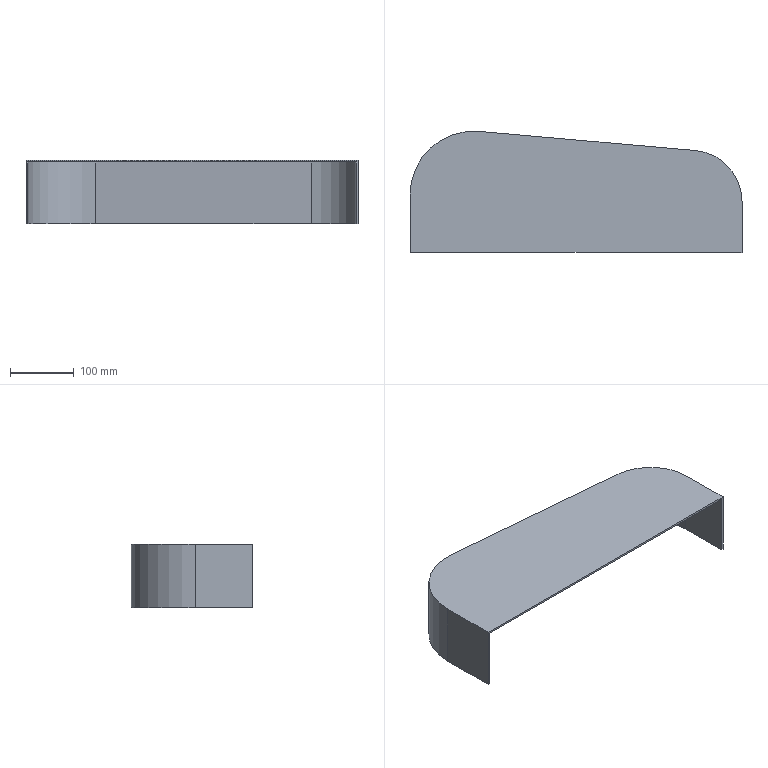Part | SolidWorks | features FlatPattern 1, SMBaseFlange 1, SheetMetal 1, Shell 1 | 1 solid | 14 faces | box 520 x 190 x 100 mm | volume 493401 mm3 | plane 10 | cylinder 4 | commonest cylinder face diameters 154 x1 160 x1 194 x1 200 x1
STEP:
#1=CARTESIAN_POINT('',(-100.,0.,-100.));
#2=VERTEX_POINT('',#1);
#3=CARTESIAN_POINT('',(-97.,0.,-100.));
#4=VERTEX_POINT('',#3);
#5=CARTESIAN_POINT('',(-100.,0.,-100.));
#6=DIRECTION('',(1.,0.,0.));
#7=VECTOR('',#6,1000.);
#8=LINE('',#5,#7);
#9=EDGE_CURVE('',#2,#4,#8,.T.);
#10=ORIENTED_EDGE('',*,*,#9,.T.);
#11=CARTESIAN_POINT('',(-97.,0.,-3.));
#12=VERTEX_POINT('',#11);
#13=CARTESIAN_POINT('',(-97.,0.,-100.));
#14=DIRECTION('',(0.,0.,1.));
#15=VECTOR('',#14,1000.);
#16=LINE('',#13,#15);
#17=EDGE_CURVE('',#4,#12,#16,.T.);
#18=ORIENTED_EDGE('',*,*,#17,.T.);
#19=CARTESIAN_POINT('',(417.,0.,-3.));
#20=VERTEX_POINT('',#19);
#21=CARTESIAN_POINT('',(0.,0.,-3.));
#22=DIRECTION('',(1.,0.,0.));
#23=VECTOR('',#22,1000.);
#24=LINE('',#21,#23);
#25=EDGE_CURVE('',#12,#20,#24,.T.);
#26=ORIENTED_EDGE('',*,*,#25,.T.);
#27=CARTESIAN_POINT('',(417.,0.,-100.));
#28=VERTEX_POINT('',#27);
#29=CARTESIAN_POINT('',(417.,0.,-100.));
#30=DIRECTION('',(0.,0.,1.));
#31=VECTOR('',#30,1000.);
#32=LINE('',#29,#31);
#33=EDGE_CURVE('',#28,#20,#32,.T.);
#34=ORIENTED_EDGE('',*,*,#33,.F.);
#35=CARTESIAN_POINT('',(420.,0.,-100.));
#36=VERTEX_POINT('',#35);
#37=CARTESIAN_POINT('',(-100.,0.,-100.));
#38=DIRECTION('',(1.,0.,0.));
#39=VECTOR('',#38,1000.);
#40=LINE('',#37,#39);
#41=EDGE_CURVE('',#28,#36,#40,.T.);
#42=ORIENTED_EDGE('',*,*,#41,.T.);
#43=CARTESIAN_POINT('',(420.,0.,0.));
#44=VERTEX_POINT('',#43);
#45=CARTESIAN_POINT('',(420.,0.,-100.));
#46=DIRECTION('',(0.,0.,1.));
#47=VECTOR('',#46,1000.);
#48=LINE('',#45,#47);
#49=EDGE_CURVE('',#36,#44,#48,.T.);
#50=ORIENTED_EDGE('',*,*,#49,.T.);
#51=CARTESIAN_POINT('',(-100.,0.,0.));
#52=VERTEX_POINT('',#51);
#53=CARTESIAN_POINT('',(-100.,0.,0.));
#54=DIRECTION('',(1.,0.,0.));
#55=VECTOR('',#54,1000.);
#56=LINE('',#53,#55);
#57=EDGE_CURVE('',#52,#44,#56,.T.);
#58=ORIENTED_EDGE('',*,*,#57,.F.);
#59=CARTESIAN_POINT('',(-100.,0.,-100.));
#60=DIRECTION('',(0.,0.,1.));
#61=VECTOR('',#60,1000.);
#62=LINE('',#59,#61);
#63=EDGE_CURVE('',#2,#52,#62,.T.);
#64=ORIENTED_EDGE('',*,*,#63,.F.);
#65=EDGE_LOOP('',(#10,#18,#26,#34,#42,#50,#58,#64));
#66=FACE_OUTER_BOUND('',#65,.T.);
#67=CARTESIAN_POINT('',(-100.,0.,-100.));
#68=DIRECTION('',(0.,-1.,0.));
#69=DIRECTION('',(1.,0.,0.));
#70=AXIS2_PLACEMENT_3D('',#67,#68,#69);
#71=PLANE('',#70);
#72=ADVANCED_FACE('',(#66),#71,.T.);
#73=CARTESIAN_POINT('',(8.812,189.611,0.));
#74=VERTEX_POINT('',#73);
#75=CARTESIAN_POINT('',(-100.,90.,0.));
#76=VERTEX_POINT('',#75);
#77=CARTESIAN_POINT('',(0.,90.,0.));
#78=DIRECTION('',(0.,0.,1.));
#79=DIRECTION('',(1.,0.,0.));
#80=AXIS2_PLACEMENT_3D('',#77,#78,#79);
#81=CIRCLE('',#80,100.);
#82=EDGE_CURVE('',#74,#76,#81,.T.);
#83=ORIENTED_EDGE('',*,*,#82,.F.);
#84=CARTESIAN_POINT('',(8.812,189.611,-100.));
#85=VERTEX_POINT('',#84);
#86=CARTESIAN_POINT('',(8.812,189.611,-100.));
#87=DIRECTION('',(0.,0.,1.));
#88=VECTOR('',#87,1000.);
#89=LINE('',#86,#88);
#90=EDGE_CURVE('',#85,#74,#89,.T.);
#91=ORIENTED_EDGE('',*,*,#90,.F.);
#92=CARTESIAN_POINT('',(-100.,90.,-100.));
#93=VERTEX_POINT('',#92);
#94=CARTESIAN_POINT('',(0.,90.,-100.));
#95=DIRECTION('',(0.,0.,1.));
#96=DIRECTION('',(1.,0.,0.));
#97=AXIS2_PLACEMENT_3D('',#94,#95,#96);
#98=CIRCLE('',#97,100.);
#99=EDGE_CURVE('',#85,#93,#98,.T.);
#100=ORIENTED_EDGE('',*,*,#99,.T.);
#101=CARTESIAN_POINT('',(-100.,90.,-100.));
#102=DIRECTION('',(0.,0.,1.));
#103=VECTOR('',#102,1000.);
#104=LINE('',#101,#103);
#105=EDGE_CURVE('',#93,#76,#104,.T.);
#106=ORIENTED_EDGE('',*,*,#105,.T.);
#107=EDGE_LOOP('',(#83,#91,#100,#106));
#108=FACE_OUTER_BOUND('',#107,.T.);
#109=CARTESIAN_POINT('',(0.,90.,-100.));
#110=DIRECTION('',(0.,0.,1.));
#111=DIRECTION('',(1.,0.,0.));
#112=AXIS2_PLACEMENT_3D('',#109,#110,#111);
#113=CYLINDRICAL_SURFACE('',#112,100.);
#114=ADVANCED_FACE('',(#108),#113,.T.);
#115=CARTESIAN_POINT('',(347.05,159.689,0.));
#116=VERTEX_POINT('',#115);
#117=CARTESIAN_POINT('',(8.812,189.611,0.));
#118=DIRECTION('',(-0.9961,0.08812,0.));
#119=VECTOR('',#118,1000.);
#120=LINE('',#117,#119);
#121=EDGE_CURVE('',#116,#74,#120,.T.);
#122=ORIENTED_EDGE('',*,*,#121,.F.);
#123=CARTESIAN_POINT('',(347.05,159.689,-100.));
#124=VERTEX_POINT('',#123);
#125=CARTESIAN_POINT('',(347.05,159.689,-100.));
#126=DIRECTION('',(0.,0.,1.));
#127=VECTOR('',#126,1000.);
#128=LINE('',#125,#127);
#129=EDGE_CURVE('',#124,#116,#128,.T.);
#130=ORIENTED_EDGE('',*,*,#129,.F.);
#131=CARTESIAN_POINT('',(8.812,189.611,-100.));
#132=DIRECTION('',(-0.9961,0.08812,0.));
#133=VECTOR('',#132,1000.);
#134=LINE('',#131,#133);
#135=EDGE_CURVE('',#124,#85,#134,.T.);
#136=ORIENTED_EDGE('',*,*,#135,.T.);
#137=ORIENTED_EDGE('',*,*,#90,.T.);
#138=EDGE_LOOP('',(#122,#130,#136,#137));
#139=FACE_OUTER_BOUND('',#138,.T.);
#140=CARTESIAN_POINT('',(8.812,189.611,-100.));
#141=DIRECTION('',(0.08812,0.9961,0.));
#142=DIRECTION('',(-0.9961,0.08812,0.));
#143=AXIS2_PLACEMENT_3D('',#140,#141,#142);
#144=PLANE('',#143);
#145=ADVANCED_FACE('',(#139),#144,.T.);
#146=CARTESIAN_POINT('',(420.,80.,0.));
#147=VERTEX_POINT('',#146);
#148=CARTESIAN_POINT('',(340.,80.,0.));
#149=DIRECTION('',(0.,0.,1.));
#150=DIRECTION('',(1.,0.,0.));
#151=AXIS2_PLACEMENT_3D('',#148,#149,#150);
#152=CIRCLE('',#151,80.);
#153=EDGE_CURVE('',#147,#116,#152,.T.);
#154=ORIENTED_EDGE('',*,*,#153,.F.);
#155=CARTESIAN_POINT('',(420.,80.,-100.));
#156=VERTEX_POINT('',#155);
#157=CARTESIAN_POINT('',(420.,80.,-100.));
#158=DIRECTION('',(0.,0.,1.));
#159=VECTOR('',#158,1000.);
#160=LINE('',#157,#159);
#161=EDGE_CURVE('',#156,#147,#160,.T.);
#162=ORIENTED_EDGE('',*,*,#161,.F.);
#163=CARTESIAN_POINT('',(340.,80.,-100.));
#164=DIRECTION('',(0.,0.,1.));
#165=DIRECTION('',(1.,0.,0.));
#166=AXIS2_PLACEMENT_3D('',#163,#164,#165);
#167=CIRCLE('',#166,80.);
#168=EDGE_CURVE('',#156,#124,#167,.T.);
#169=ORIENTED_EDGE('',*,*,#168,.T.);
#170=ORIENTED_EDGE('',*,*,#129,.T.);
#171=EDGE_LOOP('',(#154,#162,#169,#170));
#172=FACE_OUTER_BOUND('',#171,.T.);
#173=CARTESIAN_POINT('',(340.,80.,-100.));
#174=DIRECTION('',(0.,0.,1.));
#175=DIRECTION('',(1.,0.,0.));
#176=AXIS2_PLACEMENT_3D('',#173,#174,#175);
#177=CYLINDRICAL_SURFACE('',#176,80.);
#178=ADVANCED_FACE('',(#172),#177,.T.);
#179=CARTESIAN_POINT('',(420.,80.,0.));
#180=DIRECTION('',(0.,1.,0.));
#181=VECTOR('',#180,1000.);
#182=LINE('',#179,#181);
#183=EDGE_CURVE('',#44,#147,#182,.T.);
#184=ORIENTED_EDGE('',*,*,#183,.F.);
#185=ORIENTED_EDGE('',*,*,#49,.F.);
#186=CARTESIAN_POINT('',(420.,80.,-100.));
#187=DIRECTION('',(0.,1.,0.));
#188=VECTOR('',#187,1000.);
#189=LINE('',#186,#188);
#190=EDGE_CURVE('',#36,#156,#189,.T.);
#191=ORIENTED_EDGE('',*,*,#190,.T.);
#192=ORIENTED_EDGE('',*,*,#161,.T.);
#193=EDGE_LOOP('',(#184,#185,#191,#192));
#194=FACE_OUTER_BOUND('',#193,.T.);
#195=CARTESIAN_POINT('',(420.,80.,-100.));
#196=DIRECTION('',(1.,0.,0.));
#197=DIRECTION('',(0.,0.,-1.));
#198=AXIS2_PLACEMENT_3D('',#195,#196,#197);
#199=PLANE('',#198);
#200=ADVANCED_FACE('',(#194),#199,.T.);
#201=CARTESIAN_POINT('',(-100.,90.,0.));
#202=DIRECTION('',(0.,-1.,0.));
#203=VECTOR('',#202,1000.);
#204=LINE('',#201,#203);
#205=EDGE_CURVE('',#76,#52,#204,.T.);
#206=ORIENTED_EDGE('',*,*,#205,.F.);
#207=ORIENTED_EDGE('',*,*,#105,.F.);
#208=CARTESIAN_POINT('',(-100.,90.,-100.));
#209=DIRECTION('',(0.,-1.,0.));
#210=VECTOR('',#209,1000.);
#211=LINE('',#208,#210);
#212=EDGE_CURVE('',#93,#2,#211,.T.);
#213=ORIENTED_EDGE('',*,*,#212,.T.);
#214=ORIENTED_EDGE('',*,*,#63,.T.);
#215=EDGE_LOOP('',(#206,#207,#213,#214));
#216=FACE_OUTER_BOUND('',#215,.T.);
#217=CARTESIAN_POINT('',(-100.,90.,-100.));
#218=DIRECTION('',(-1.,0.,0.));
#219=DIRECTION('',(0.,0.,1.));
#220=AXIS2_PLACEMENT_3D('',#217,#218,#219);
#221=PLANE('',#220);
#222=ADVANCED_FACE('',(#216),#221,.T.);
#223=ORIENTED_EDGE('',*,*,#41,.F.);
#224=CARTESIAN_POINT('',(417.,80.,-100.));
#225=VERTEX_POINT('',#224);
#226=CARTESIAN_POINT('',(417.,90.,-100.));
#227=DIRECTION('',(0.,1.,0.));
#228=VECTOR('',#227,1000.);
#229=LINE('',#226,#228);
#230=EDGE_CURVE('',#28,#225,#229,.T.);
#231=ORIENTED_EDGE('',*,*,#230,.T.);
#232=CARTESIAN_POINT('',(346.785,156.7,-100.));
#233=VERTEX_POINT('',#232);
#234=CARTESIAN_POINT('',(340.,80.,-100.));
#235=DIRECTION('',(0.,0.,1.));
#236=DIRECTION('',(1.,0.,0.));
#237=AXIS2_PLACEMENT_3D('',#234,#235,#236);
#238=CIRCLE('',#237,77.);
#239=EDGE_CURVE('',#225,#233,#238,.T.);
#240=ORIENTED_EDGE('',*,*,#239,.T.);
#241=CARTESIAN_POINT('',(8.548,186.623,-100.));
#242=VERTEX_POINT('',#241);
#243=CARTESIAN_POINT('',(8.548,186.623,-100.));
#244=DIRECTION('',(-0.9961,0.08812,0.));
#245=VECTOR('',#244,1000.);
#246=LINE('',#243,#245);
#247=EDGE_CURVE('',#233,#242,#246,.T.);
#248=ORIENTED_EDGE('',*,*,#247,.T.);
#249=CARTESIAN_POINT('',(-97.,90.,-100.));
#250=VERTEX_POINT('',#249);
#251=CARTESIAN_POINT('',(0.,90.,-100.));
#252=DIRECTION('',(0.,0.,1.));
#253=DIRECTION('',(1.,0.,0.));
#254=AXIS2_PLACEMENT_3D('',#251,#252,#253);
#255=CIRCLE('',#254,97.);
#256=EDGE_CURVE('',#242,#250,#255,.T.);
#257=ORIENTED_EDGE('',*,*,#256,.T.);
#258=CARTESIAN_POINT('',(-97.,90.,-100.));
#259=DIRECTION('',(0.,-1.,0.));
#260=VECTOR('',#259,1000.);
#261=LINE('',#258,#260);
#262=EDGE_CURVE('',#250,#4,#261,.T.);
#263=ORIENTED_EDGE('',*,*,#262,.T.);
#264=ORIENTED_EDGE('',*,*,#9,.F.);
#265=ORIENTED_EDGE('',*,*,#212,.F.);
#266=ORIENTED_EDGE('',*,*,#99,.F.);
#267=ORIENTED_EDGE('',*,*,#135,.F.);
#268=ORIENTED_EDGE('',*,*,#168,.F.);
#269=ORIENTED_EDGE('',*,*,#190,.F.);
#270=EDGE_LOOP('',(#223,#231,#240,#248,#257,#263,#264,#265,#266,#267,#268,#269));
#271=FACE_OUTER_BOUND('',#270,.T.);
#272=CARTESIAN_POINT('',(0.,90.,-100.));
#273=DIRECTION('',(0.,0.,1.));
#274=DIRECTION('',(1.,0.,0.));
#275=AXIS2_PLACEMENT_3D('',#272,#273,#274);
#276=PLANE('',#275);
#277=ADVANCED_FACE('',(#271),#276,.F.);
#278=ORIENTED_EDGE('',*,*,#82,.T.);
#279=ORIENTED_EDGE('',*,*,#205,.T.);
#280=ORIENTED_EDGE('',*,*,#57,.T.);
#281=ORIENTED_EDGE('',*,*,#183,.T.);
#282=ORIENTED_EDGE('',*,*,#153,.T.);
#283=ORIENTED_EDGE('',*,*,#121,.T.);
#284=EDGE_LOOP('',(#278,#279,#280,#281,#282,#283));
#285=FACE_OUTER_BOUND('',#284,.T.);
#286=CARTESIAN_POINT('',(0.,90.,0.));
#287=DIRECTION('',(0.,0.,1.));
#288=DIRECTION('',(1.,0.,0.));
#289=AXIS2_PLACEMENT_3D('',#286,#287,#288);
#290=PLANE('',#289);
#291=ADVANCED_FACE('',(#285),#290,.T.);
#292=CARTESIAN_POINT('',(8.548,186.623,-3.));
#293=VERTEX_POINT('',#292);
#294=CARTESIAN_POINT('',(-97.,90.,-3.));
#295=VERTEX_POINT('',#294);
#296=CARTESIAN_POINT('',(0.,90.,-3.));
#297=DIRECTION('',(0.,0.,1.));
#298=DIRECTION('',(1.,0.,0.));
#299=AXIS2_PLACEMENT_3D('',#296,#297,#298);
#300=CIRCLE('',#299,97.);
#301=EDGE_CURVE('',#293,#295,#300,.T.);
#302=ORIENTED_EDGE('',*,*,#301,.T.);
#303=CARTESIAN_POINT('',(-97.,90.,-100.));
#304=DIRECTION('',(0.,0.,1.));
#305=VECTOR('',#304,1000.);
#306=LINE('',#303,#305);
#307=EDGE_CURVE('',#250,#295,#306,.T.);
#308=ORIENTED_EDGE('',*,*,#307,.F.);
#309=ORIENTED_EDGE('',*,*,#256,.F.);
#310=CARTESIAN_POINT('',(8.548,186.623,-100.));
#311=DIRECTION('',(0.,0.,1.));
#312=VECTOR('',#311,1000.);
#313=LINE('',#310,#312);
#314=EDGE_CURVE('',#242,#293,#313,.T.);
#315=ORIENTED_EDGE('',*,*,#314,.T.);
#316=EDGE_LOOP('',(#302,#308,#309,#315));
#317=FACE_OUTER_BOUND('',#316,.T.);
#318=CARTESIAN_POINT('',(0.,90.,-100.));
#319=DIRECTION('',(0.,0.,1.));
#320=DIRECTION('',(1.,0.,0.));
#321=AXIS2_PLACEMENT_3D('',#318,#319,#320);
#322=CYLINDRICAL_SURFACE('',#321,97.);
#323=ADVANCED_FACE('',(#317),#322,.F.);
#324=CARTESIAN_POINT('',(346.785,156.7,-3.));
#325=VERTEX_POINT('',#324);
#326=CARTESIAN_POINT('',(8.548,186.623,-3.));
#327=DIRECTION('',(-0.9961,0.08812,0.));
#328=VECTOR('',#327,1000.);
#329=LINE('',#326,#328);
#330=EDGE_CURVE('',#325,#293,#329,.T.);
#331=ORIENTED_EDGE('',*,*,#330,.T.);
#332=ORIENTED_EDGE('',*,*,#314,.F.);
#333=ORIENTED_EDGE('',*,*,#247,.F.);
#334=CARTESIAN_POINT('',(346.785,156.7,-100.));
#335=DIRECTION('',(0.,0.,1.));
#336=VECTOR('',#335,1000.);
#337=LINE('',#334,#336);
#338=EDGE_CURVE('',#233,#325,#337,.T.);
#339=ORIENTED_EDGE('',*,*,#338,.T.);
#340=EDGE_LOOP('',(#331,#332,#333,#339));
#341=FACE_OUTER_BOUND('',#340,.T.);
#342=CARTESIAN_POINT('',(8.548,186.623,-100.));
#343=DIRECTION('',(0.08812,0.9961,0.));
#344=DIRECTION('',(-0.9961,0.08812,0.));
#345=AXIS2_PLACEMENT_3D('',#342,#343,#344);
#346=PLANE('',#345);
#347=ADVANCED_FACE('',(#341),#346,.F.);
#348=CARTESIAN_POINT('',(417.,80.,-3.));
#349=VERTEX_POINT('',#348);
#350=CARTESIAN_POINT('',(340.,80.,-3.));
#351=DIRECTION('',(0.,0.,1.));
#352=DIRECTION('',(1.,0.,0.));
#353=AXIS2_PLACEMENT_3D('',#350,#351,#352);
#354=CIRCLE('',#353,77.);
#355=EDGE_CURVE('',#349,#325,#354,.T.);
#356=ORIENTED_EDGE('',*,*,#355,.T.);
#357=ORIENTED_EDGE('',*,*,#338,.F.);
#358=ORIENTED_EDGE('',*,*,#239,.F.);
#359=CARTESIAN_POINT('',(417.,80.,-100.));
#360=DIRECTION('',(0.,0.,1.));
#361=VECTOR('',#360,1000.);
#362=LINE('',#359,#361);
#363=EDGE_CURVE('',#225,#349,#362,.T.);
#364=ORIENTED_EDGE('',*,*,#363,.T.);
#365=EDGE_LOOP('',(#356,#357,#358,#364));
#366=FACE_OUTER_BOUND('',#365,.T.);
#367=CARTESIAN_POINT('',(340.,80.,-100.));
#368=DIRECTION('',(0.,0.,1.));
#369=DIRECTION('',(1.,0.,0.));
#370=AXIS2_PLACEMENT_3D('',#367,#368,#369);
#371=CYLINDRICAL_SURFACE('',#370,77.);
#372=ADVANCED_FACE('',(#366),#371,.F.);
#373=CARTESIAN_POINT('',(417.,90.,-3.));
#374=DIRECTION('',(0.,1.,0.));
#375=VECTOR('',#374,1000.);
#376=LINE('',#373,#375);
#377=EDGE_CURVE('',#20,#349,#376,.T.);
#378=ORIENTED_EDGE('',*,*,#377,.T.);
#379=ORIENTED_EDGE('',*,*,#363,.F.);
#380=ORIENTED_EDGE('',*,*,#230,.F.);
#381=ORIENTED_EDGE('',*,*,#33,.T.);
#382=EDGE_LOOP('',(#378,#379,#380,#381));
#383=FACE_OUTER_BOUND('',#382,.T.);
#384=CARTESIAN_POINT('',(417.,80.,-100.));
#385=DIRECTION('',(1.,0.,0.));
#386=DIRECTION('',(0.,0.,-1.));
#387=AXIS2_PLACEMENT_3D('',#384,#385,#386);
#388=PLANE('',#387);
#389=ADVANCED_FACE('',(#383),#388,.F.);
#390=CARTESIAN_POINT('',(-97.,90.,-3.));
#391=DIRECTION('',(0.,-1.,0.));
#392=VECTOR('',#391,1000.);
#393=LINE('',#390,#392);
#394=EDGE_CURVE('',#295,#12,#393,.T.);
#395=ORIENTED_EDGE('',*,*,#394,.T.);
#396=ORIENTED_EDGE('',*,*,#17,.F.);
#397=ORIENTED_EDGE('',*,*,#262,.F.);
#398=ORIENTED_EDGE('',*,*,#307,.T.);
#399=EDGE_LOOP('',(#395,#396,#397,#398));
#400=FACE_OUTER_BOUND('',#399,.T.);
#401=CARTESIAN_POINT('',(-97.,90.,-100.));
#402=DIRECTION('',(-1.,0.,0.));
#403=DIRECTION('',(0.,0.,1.));
#404=AXIS2_PLACEMENT_3D('',#401,#402,#403);
#405=PLANE('',#404);
#406=ADVANCED_FACE('',(#400),#405,.F.);
#407=ORIENTED_EDGE('',*,*,#301,.F.);
#408=ORIENTED_EDGE('',*,*,#330,.F.);
#409=ORIENTED_EDGE('',*,*,#355,.F.);
#410=ORIENTED_EDGE('',*,*,#377,.F.);
#411=ORIENTED_EDGE('',*,*,#25,.F.);
#412=ORIENTED_EDGE('',*,*,#394,.F.);
#413=EDGE_LOOP('',(#407,#408,#409,#410,#411,#412));
#414=FACE_OUTER_BOUND('',#413,.T.);
#415=CARTESIAN_POINT('',(0.,90.,-3.));
#416=DIRECTION('',(0.,0.,1.));
#417=DIRECTION('',(1.,0.,0.));
#418=AXIS2_PLACEMENT_3D('',#415,#416,#417);
#419=PLANE('',#418);
#420=ADVANCED_FACE('',(#414),#419,.F.);
#421=CLOSED_SHELL('',(#72,#114,#145,#178,#200,#222,#277,#291,#323,#347,#372,#389,#406,#420));
#422=MANIFOLD_SOLID_BREP('',#421);
#423=CARTESIAN_POINT('',(0.,0.,0.));
#424=DIRECTION('',(0.,0.,1.));
#425=DIRECTION('',(1.,0.,0.));
#426=AXIS2_PLACEMENT_3D('',#423,#424,#425);
#427=(LENGTH_UNIT()NAMED_UNIT(*)SI_UNIT(.MILLI.,.METRE.));
#428=UNCERTAINTY_MEASURE_WITH_UNIT(LENGTH_MEASURE(0.00001),#427,'','');
#429=(NAMED_UNIT(*)PLANE_ANGLE_UNIT()SI_UNIT($,.RADIAN.));
#430=(NAMED_UNIT(*)SI_UNIT($,.STERADIAN.)SOLID_ANGLE_UNIT());
#431=(GEOMETRIC_REPRESENTATION_CONTEXT(3)GLOBAL_UNCERTAINTY_ASSIGNED_CONTEXT((#428))GLOBAL_UNIT_ASSIGNED_CONTEXT((#427,#429,#430))REPRESENTATION_CONTEXT('',''));
#432=ADVANCED_BREP_SHAPE_REPRESENTATION('',(#422,#426),#431);